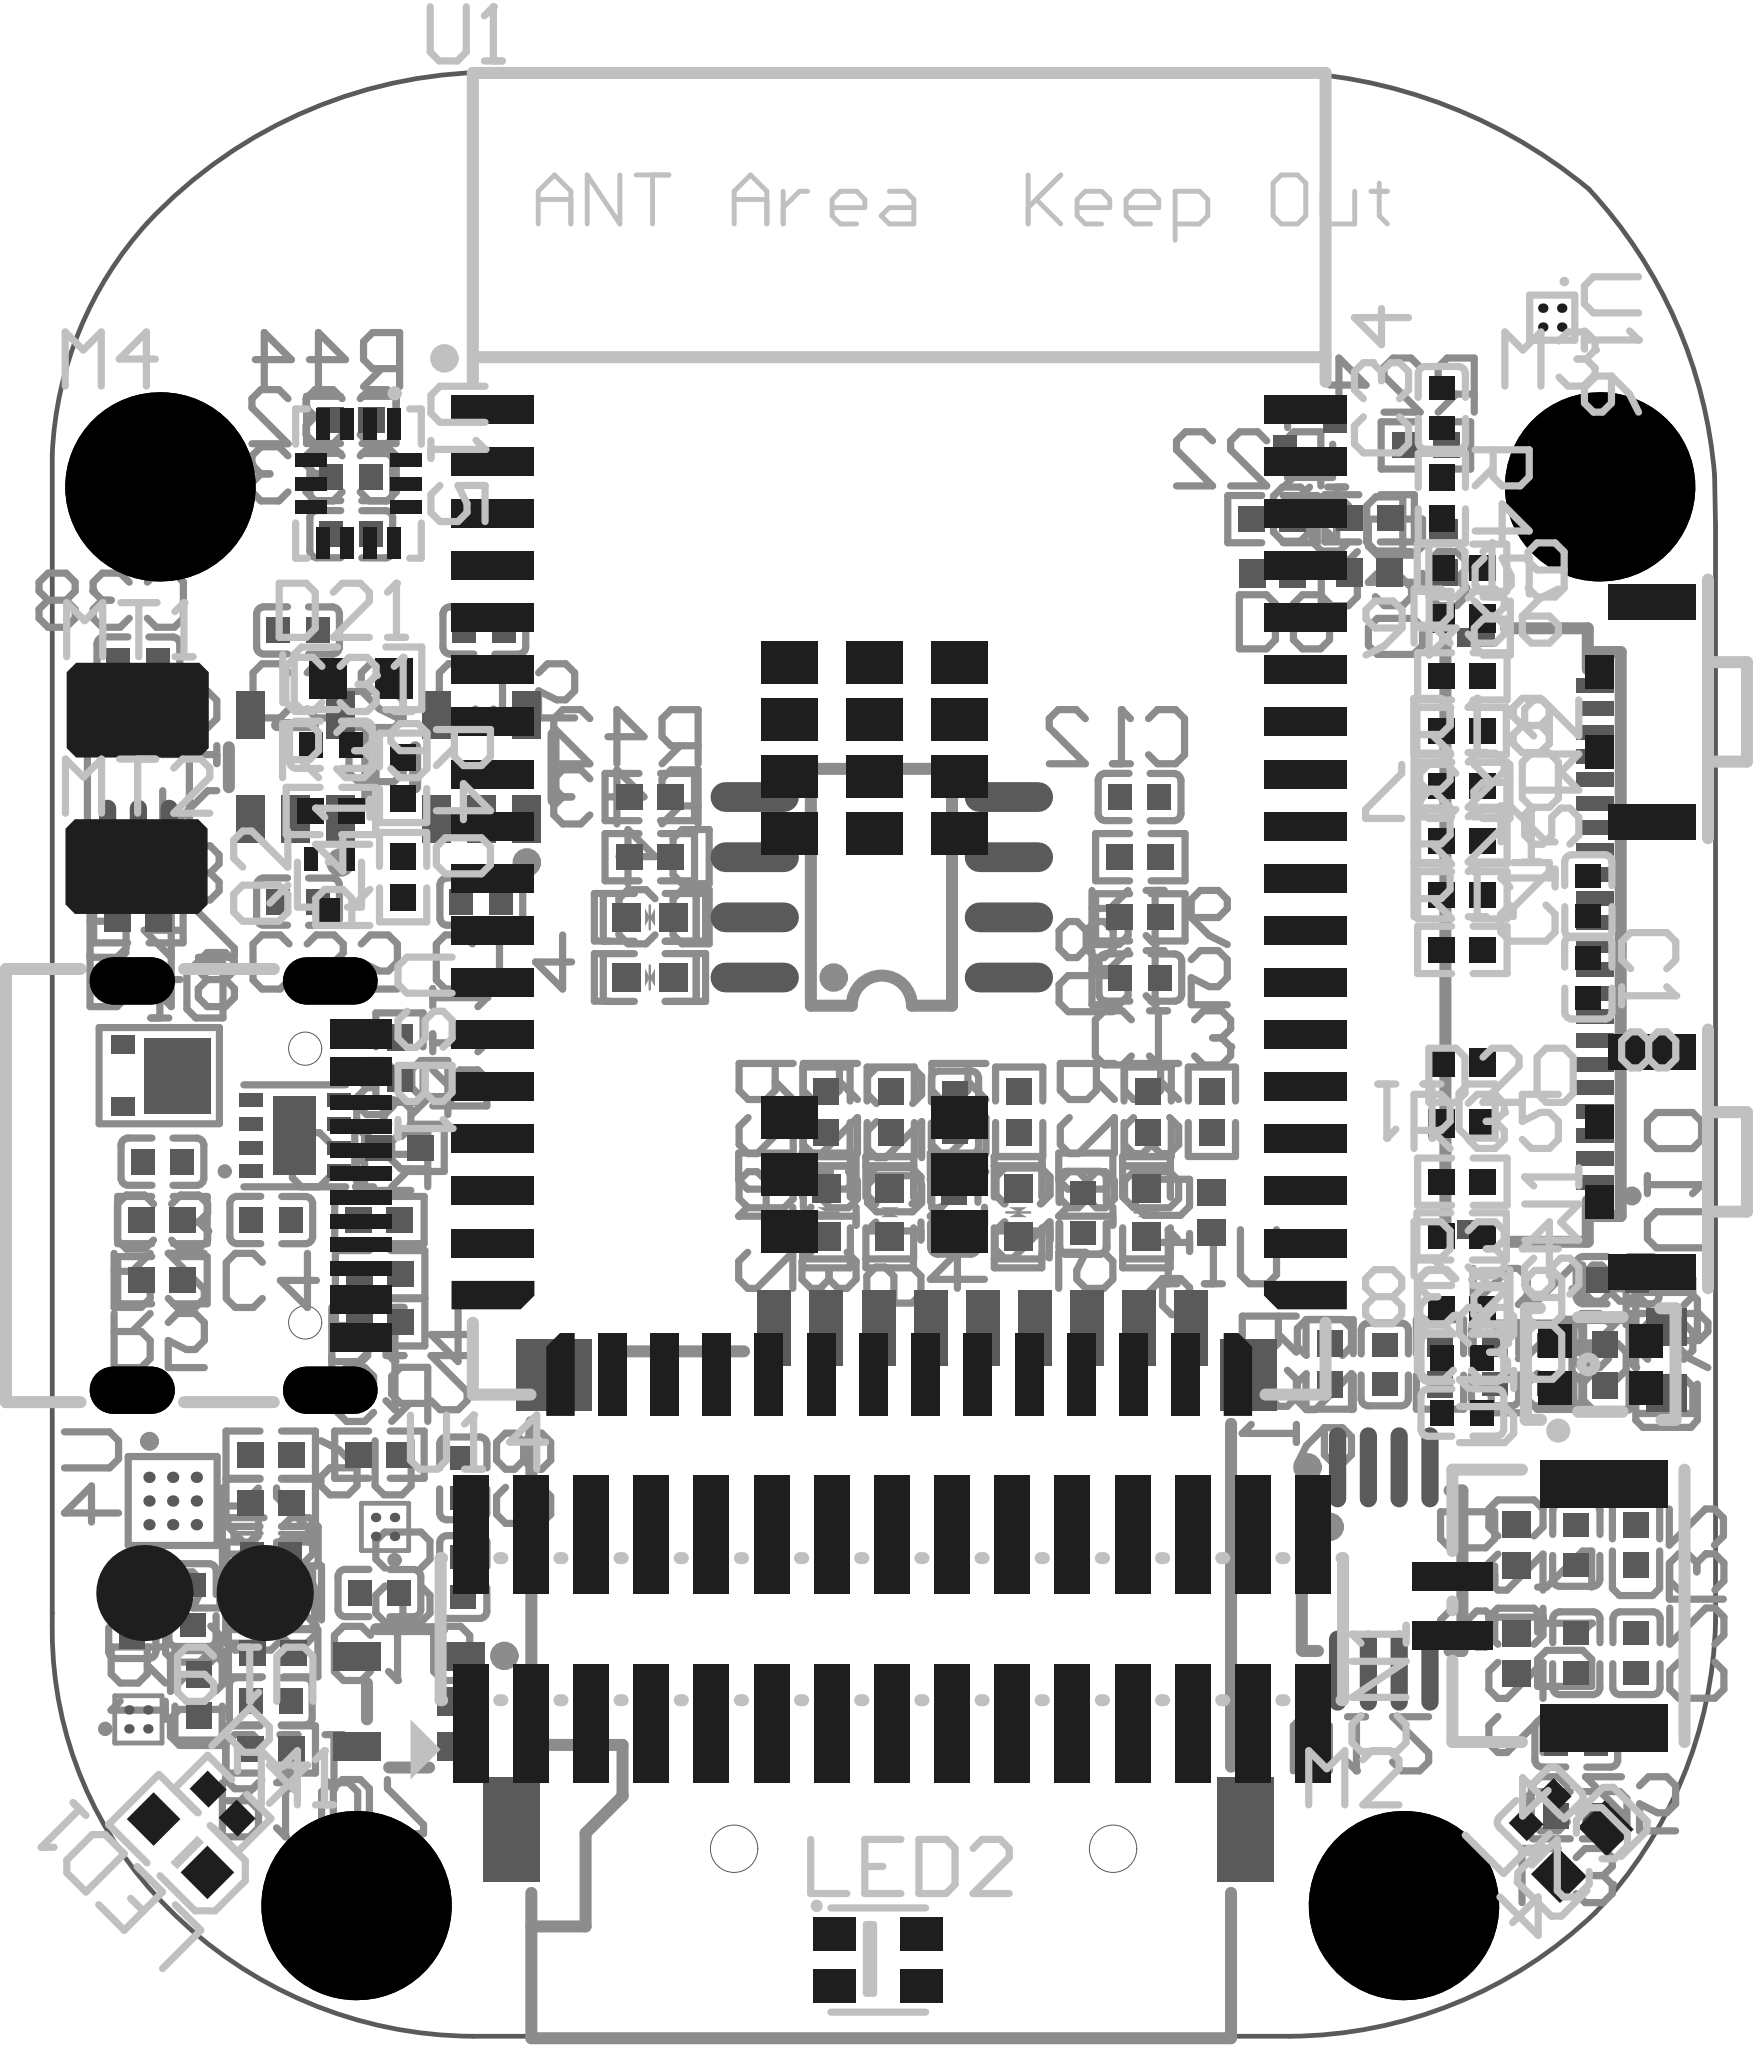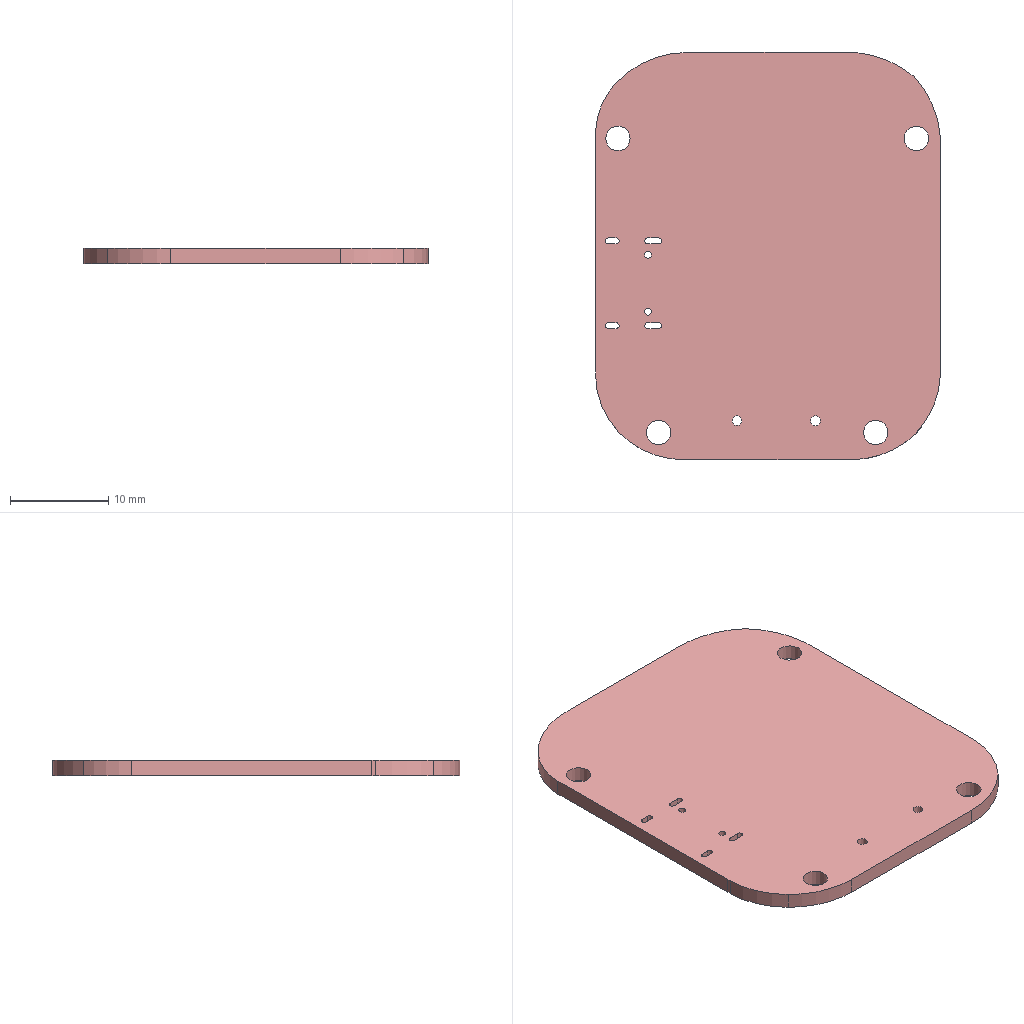Circuit board layout | Altium Designer | box 35.1 x 41.5 x 1.6 mm
Layer stack:
# Altium Designer layer stack of  (unit mm; dielectric type: 0 none, 1 core, 2 prepreg, 3 surface material)
index,name,kind,layer,copper_thickness_mm,dielectric_type,dielectric_thickness_mm,dielectric_material,dielectric_constant
0,Top Paste Mask Layer,other,,,,,,
1,Top Silkscreen Layer,other,,,,,,
2,Top Solder Mask Layer,dielectric,,,3,0.01,,3.3
3,Top Layer,copper,Top Layer,0.035,,,,
4,Dielectric1,dielectric,,,3,1.51,FR4,4.5
5,Bottom Layer,copper,Bottom Layer,0.035,,,,
6,Bottom Solder Mask Layer,dielectric,,,3,0.01,,3.3
7,Bottom Silkscreen Layer,other,,,,,,
8,Bottom Paste Mask Layer,other,,,,,,
# drill layer pairs: low layer,high layer
drill_pair,Top Layer,Bottom Layer
Part placement:
Designator,Comment,Layer,Footprint,Center-X(mm),Center-Y(mm),Rotation
C1,1uF,BottomLayer,C0402,98.943,93.625,270
C2,4.7uF,BottomLayer,C0402,98.926,93.625,270
C3,1uF,BottomLayer,C0402,79.502,94.704,0
C4,4.7uF,BottomLayer,C0402,81.799,93.472,0
C5,10uF,BottomLayer,C0402,78.867,85.09,90
C6,4.7uF,BottomLayer,C0402,80.137,85.344,90
C7,1uF,BottomLayer,C0402,81.839,85.344,180
C8,1uF,BottomLayer,C0402,85.852,88.019,90
C9,1uF,BottomLayer,C0402,85.852,85.936,270
C10,1uF,BottomLayer,C0402,84.082,85.598,0
C11,1uF,BottomLayer,C0402,81.788,83.312,0
C12,1uF,BottomLayer,C0402,100.128,102.402,180
C13,100nF,BottomLayer,C0402,100.144,98.592,0
C14,1uF,BottomLayer,C0402,86.233,100.194,0
C15,1uF,BottomLayer,C0402,86.297,105.918,0
C16,1uF,BottomLayer,C0402,110.218,92.202,0
C17,100nF,TopLayer,C0402,109.601,100.31,90
C18,4.7uF,TopLayer,C0402,109.601,98.59,270
C19,1uF,BottomLayer,C0402,96.216,93.625,270
C20,100nF,BottomLayer,C0402,96.231,95.743,270
C21,330pF,BottomLayer,C0402,109.347,86.614,270
C22,330pF,BottomLayer,C0402,109.347,84.328,270
C23,330pF,BottomLayer,C0402,110.617,84.328,90
C24,100nF,TopLayer,C0402,108.585,81.026,225
C25,22uF,BottomLayer,C0402,109.347,82.423,0
C26,1uF,BottomLayer,C0402,105.304,90.424,270
C27,100nF,BottomLayer,C0402,107.633,90.424,90
C28,100nF,BottomLayer,C0402,108.798,90.424,90
C29,4.7uF,TopLayer,C0402,106.942,90.563,0
C30,10nF,TopLayer,C0402,106.942,89.408,0
C31,4.7uF,TopLayer,C0402,83.058,103.505,0
C32,100nF,BottomLayer,C0402,83.488,109.157,180
C33,100nF,BottomLayer,C0402,83.488,107.95,180
C34,100nF,TopLayer,C0402,106.509,110.617,90
CN1,A1257WR-S-2P,TopLayer,CONN-SMD_A1257WR-S-2P,108.331,85.328,90
D1,PTVSHC3N18VU,BottomLayer,DFN-3_L2.0-W2.0-P1.30-BR,79.248,96.52,180
D2,PESDHC2FD12VU,BottomLayer,DFN1006-2L-RD,81.788,86.36,0
D3,,BottomLayer,D0402-BI,89.789,98.592,180
D4,,BottomLayer,D0402-BI,89.789,99.862,180
D8,ESD5451N,BottomLayer,DFN1006-2L-BI,102.934,107.125,0
D9,ESD5451N,BottomLayer,DFN1006-2L-BI,104.984,107.143,180
D10,ESD5451N,BottomLayer,DFN1006-2L-BI,106.553,107.569,270
D11,ESD5451N,TopLayer,DFN1006-2L-BI,106.934,96.796,180
D12,,BottomLayer,D0402-BI,93.519,93.633,270
D13,,BottomLayer,D0402-BI,94.855,93.633,270
D14,,BottomLayer,D0402-BI,97.565,93.633,270
D15,,BottomLayer,D0402-BI,100.275,93.633,270
D16,ESD5451N,BottomLayer,DFN1006-2L-BI,101.636,93.633,270
D17,ESD5451N,BottomLayer,DFN1006-2L-BI,108.077,84.328,90
D18,ESD5451N,BottomLayer,DFN1006-2L-BI,108.077,86.614,270
D19,ESD5451N,TopLayer,DFN1006-2L-BI,106.934,106.172,0
D20,ESD5451N,TopLayer,DFN1006-2L-BI,106.934,95.505,0
D21,CD4148WTP,TopLayer,D0603-RD,83.693,104.902,0
L2,,BottomLayer,L0402,110.617,86.614,90
L3,,BottomLayer,L0402,109.347,80.899,0
L4,,TopLayer,L0603,109.474,80.137,45
L5,,BottomLayer,L0603,111.252,90.52,270
LED1,,TopLayer,LED0603-RD_GREEN,79.883,80.264,135
LED2,WS2812B-2020,TopLayer,LED-SMD_4P-L2.0-W2.0-TL_WS2812B-2020,94.613,77.851,0
Q1,CJ3134K KF,BottomLayer,SOT-723_L1.2-W0.8-P0.40-LS1.2-BR,103.729,109.825,0
Q2,CJ3134K KF,TopLayer,SOT-723_L1.2-W0.8-P0.40-LS1.2-BR,83.028,100.554,90
R1,100kΩ,BottomLayer,R0402,80.264,83.439,270
R2,510kΩ,BottomLayer,R0402,79.502,93.472,0
R3,20kΩ,BottomLayer,R0402,84.506,94.996,180
R4,4.7kΩ,TopLayer,R0402,80.772,81.153,315
R5,100kΩ,BottomLayer,R0402,79.502,92.202,0
R6,100kΩ,BottomLayer,R0402,81.839,84.328,180
R7,2.2kΩ,BottomLayer,R0402,81.788,88.519,0
R8,2.2kΩ,BottomLayer,R0402,81.788,87.503,0
R9,5.1MΩ,BottomLayer,R0402,84.082,88.519,180
R10,5.1MΩ,BottomLayer,R0402,81.788,82.296,0
R11,5.1kΩ,BottomLayer,R0402,84.506,96.901,90
R12,5.1kΩ,BottomLayer,R0402,84.097,91.313,0
R13,390kΩ,BottomLayer,R0402,84.082,93.472,180
R14,510kΩ,BottomLayer,R0402,84.097,92.329,0
R15,100Ω,BottomLayer,R0402,100.144,99.862,0
R16,100Ω,BottomLayer,R0402,100.144,101.132,0
R17,22Ω,TopLayer,R0402,106.942,99.174,0
R18,22Ω,TopLayer,R0402,106.942,102.639,0
R19,22Ω,TopLayer,R0402,106.942,102.639,0
R20,22Ω,TopLayer,R0402,106.942,101.484,0
R21,22Ω,TopLayer,R0402,106.942,100.329,0
R22,2.2kΩ,BottomLayer,R0402,102.934,108.268,180
R23,2.2kΩ,BottomLayer,R0402,104.984,108.286,0
R24,2.2kΩ,BottomLayer,R0402,106.172,109.825,180
R25,22Ω,BottomLayer,R0402,94.875,95.758,270
R27,22Ω,BottomLayer,R0402,97.587,95.758,270
R28,22Ω,BottomLayer,R0402,100.299,95.758,270
R29,22Ω,BottomLayer,R0402,93.519,95.758,270
R30,22Ω,BottomLayer,R0402,101.655,95.758,270
R31,5.1MΩ,BottomLayer,R0402,104.14,90.424,270
R32,43.2kΩ,BottomLayer,R0402,106.469,90.424,90
R33,43.2kΩ,BottomLayer,R0402,109.962,90.409,90
R34,1kΩ,TopLayer,R0402,106.942,91.591,0
R35,5.1kΩ,TopLayer,R0402,106.942,94.282,0
R36,5.1kΩ,TopLayer,R0402,106.942,104.949,0
R37,15kΩ,TopLayer,R0402,106.926,103.794,180
R38,15kΩ,TopLayer,R0402,106.926,93.127,180
R39,5.1Ω,TopLayer,R0402,83.058,102.108,0
R40,1.5MΩ,TopLayer,R0402,84.582,102.807,270
R41,1kΩ,TopLayer,R0402,84.582,100.711,90
R42,22Ω,BottomLayer,R0402,89.789,102.402,180
R43,22Ω,BottomLayer,R0402,89.789,101.132,180
R44,2.2kΩ,BottomLayer,R0402,83.488,110.363,180
R45,2.2kΩ,TopLayer,R0402,106.509,108.712,270
R46,2.2kΩ,TopLayer,R0402,106.934,107.243,180
SW1,,TopLayer,KEY-SMD_GT-TC191A-H026-L60,110.389,94.7,90
SW2,,TopLayer,KEY-SMD_GT-TC191A-H026-L60,110.389,104.2,90
U1,,TopLayer,COMM-SMD_L27.9-W18.0-P1.10_SF32LB52-MOD-1-N16R8,95.054,100.384,0
U2,LP5240HVF,BottomLayer,WLCSP-4_L0.8-W0.8-R2-C2-P0.40-BL,78.994,82.931,90
U3,LP5305AQVF,BottomLayer,DFN-8_L2.0-W2.0-P0.50-BL-EP,82.296,95.25,90
U4,AW32001ECSR,BottomLayer,WLCSP-9_L1.7-W1.7-R3-C3-P0.50-TL,79.718,87.541,270
U6,LP5240HVF,BottomLayer,WLCSP-4_L0.8-W0.8-R2-C2-P0.40-BL,84.201,86.994,180
U7,ETA5055V330DS2F,BottomLayer,SOT-23-5_L2.9-W1.6-P0.95-LS2.8-BR,84.709,83.312,0
U8,CH340N,BottomLayer,SOP-8_L4.9-W3.9-P1.27-LS6.0-BL,94.687,100.497,90
U9,ETA5055V330DS2F,BottomLayer,SOT-23-5_L2.9-W1.6-P0.95-LS2.8-BR,86.233,103.031,270
U10,AFH34-S22FIA-1H,BottomLayer,FPC-SMD_22P-P0.50_JS_AFH34-S22FIA-1H,108.489,99.513,90
U11,TF-115Y-ACP9,BottomLayer,SIM-SMD_TF-115Y-BCP9,94.644,85.9,180
U12,NS4150B,BottomLayer,MSOP-8_L3.0-W3.0-P0.65-LS5.0-BL,105.283,86.106,0
U13,LMA2718T421-OA5,TopLayer,MIC-SMD_4P-L2.8-W1.9-P1.01-TL,109.855,90.424,90
U14,XDZ127-2-15-S-1.0-G1,TopLayer,HDR-SMD_30P-P1.27-V-M-R2-C15-LS5.5_1,94.899,84.836,0
U15,LSM6DS3TR-C,TopLayer,LGA-14_L3.0-W2.5-P0.50-TL,83.64,109.019,270
U16,MMC5603NJ,TopLayer,FLIPCHIP-4_L0.8-W0.8-R2-C2-P0.40-TL,108.839,112.522,270
U17,ETA5055V330DS2F,BottomLayer,SOT-23-5_L2.9-W1.6-P0.95-LS2.8-BR,82.301,103.031,270
USB1,KH-TYPE-C-16P,TopLayer,USB-C-SMD_KH-TYPE-C-16P,81.28,94.2,270
C35,1uF,BottomLayer,C0402,82.364,100.194,0
C36,1uF,BottomLayer,C0402,82.364,105.918,0
C38,100nF,BottomLayer,C0402,78.994,105.283,180
R47,5.1MΩ,BottomLayer,R0402,78.994,100.863,0
R48,22Ω,BottomLayer,R0402,78.994,99.822,0
U18,LTR-303ALS-01,BottomLayer,TDFN-6_L2.0-W2.0-P0.65-BL,78.994,102.921,0
U19,,TopLayer,焊盘,80.391,85.598,180
M1,M2-TH,TopLayer,M2_TH_4_2.5MM,83.589,79,0
M2,M2-TH,TopLayer,M2_TH_4_2.5MM,105.699,79,0
M3,M2-TH,TopLayer,M2_TH_4_2.5MM,109.839,108.95,0
M4,M2-TH,TopLayer,M2_TH_4_2.5MM,79.449,108.95,0
MT1,,TopLayer,TP-3x2MM,78.98,104.236,0
MT2,,TopLayer,TP-3x2MM,78.955,100.934,0
Pad and via stacks:
# Altium Designer via and pad stacks of  (unit mm). Each distinct definition once, with the count of objects using it.
# via: kind,start_layer,end_layer,hole_mm,diameter_mm,mode(0 simple;1 top-mid-bottom;2 full stack),diameter_per_layer,count,example_net
# pad: kind,layer,hole_mm,hole_type(0 round;1 square;2 slot),plating,top_size,top_shape(1 round;2 rect;3 octagon;9 rounded rect),mid_size,bottom_size,mode,footprint,size_per_layer,count,example
pad,Bottom Layer,0,0,plated,0.5x0.54,2,0.5x0.54,0.5x0.54,0,C0402,,60,C1.2
pad,Bottom Layer,0,0,plated,1.6x1.4,2,1.6x1.4,1.6x1.4,0,DFN-3_L2.0-W2.0-P1.30-BR,,1,D1.3
pad,Bottom Layer,0,0,plated,0.4x0.5,2,0.4x0.5,0.4x0.5,0,DFN-3_L2.0-W2.0-P1.30-BR,,2,D1.2
pad,Bottom Layer,0,0,plated,0.5x0.6,2,0.5x0.6,0.5x0.6,0,DFN1006-2L-RD,,2,D2.1
pad,Bottom Layer,0,0,plated,0.6x0.6,2,0.6x0.6,0.6x0.6,0,D0402-BI,,12,D3.1
pad,Bottom Layer,0,0,plated,0.55x0.6,2,0.55x0.6,0.55x0.6,0,DFN1006-2L-BI,,12,D8.1
pad,Bottom Layer,0,0,plated,0.54x0.54,2,0.54x0.54,0.54x0.54,0,L0402,,4,L2.2
pad,Bottom Layer,0,0,plated,0.8x0.864,2,0.8x0.864,0.8x0.864,0,L0603,,2,L5.1
pad,Bottom Layer,0,0,plated,0.489x0.294,2,0.489x0.294,0.489x0.294,0,SOT-723_L1.2-W0.8-P0.40-LS1.2-BR,,2,Q1.1
pad,Bottom Layer,0,0,plated,0.489x0.434,2,0.489x0.434,0.489x0.434,0,SOT-723_L1.2-W0.8-P0.40-LS1.2-BR,,1,Q1.3
pad,Bottom Layer,0,0,plated,0.5657x0.54,2,0.5657x0.54,0.5657x0.54,0,R0402,,62,R1.2
pad,Bottom Layer,0,0,plated,0.2x0.2,1,0.2x0.2,0.2x0.2,0,WLCSP-4_L0.8-W0.8-R2-C2-P0.40-BL,,8,U2.A1
pad,Bottom Layer,0,0,plated,0.28x0.505,2,0.28x0.505,0.28x0.505,0,DFN-8_L2.0-W2.0-P0.50-BL-EP,,8,U3.1
pad,Bottom Layer,0,0,plated,1.65x0.9,2,1.65x0.9,1.65x0.9,0,DFN-8_L2.0-W2.0-P0.50-BL-EP,,1,U3.9
pad,Bottom Layer,0,0,plated,0.24x0.24,1,0.24x0.24,0.24x0.24,0,WLCSP-9_L1.7-W1.7-R3-C3-P0.50-TL,,9,U4.A1
pad,Bottom Layer,0,0,plated,0.6x1,2,0.6x1,0.6x1,0,SOT-23-5_L2.9-W1.6-P0.95-LS2.8-BR,,15,U7.2
pad,Bottom Layer,0,0,plated,0.63x1.865,1,0.63x1.865,0.63x1.865,0,SOP-8_L4.9-W3.9-P1.27-LS6.0-BL,,8,U8.1
pad,Bottom Layer,0,0,plated,0.4x0.8,2,0.4x0.8,0.4x0.8,0,FPC-SMD_22P-P0.50_JS_AFH34-S22FIA-1H,,2,U10.24
pad,Bottom Layer,0,0,plated,0.3x0.8,2,0.3x0.8,0.3x0.8,0,FPC-SMD_22P-P0.50_JS_AFH34-S22FIA-1H,,22,U10.22
pad,Bottom Layer,0,0,plated,0.7x1.6,2,0.7x1.6,0.7x1.6,0,SIM-SMD_TF-115Y-BCP9,,9,U11.1
pad,Bottom Layer,0,0,plated,1.2x1.5,2,1.2x1.5,1.2x1.5,0,SIM-SMD_TF-115Y-BCP9,,1,U11.10
pad,Bottom Layer,0,0,plated,1.6x1.5,2,1.6x1.5,1.6x1.5,0,SIM-SMD_TF-115Y-BCP9,,1,U11.11
pad,Bottom Layer,0,0,plated,1.2x2.2,2,1.2x2.2,1.2x2.2,0,SIM-SMD_TF-115Y-BCP9,,2,U11.12
pad,Bottom Layer,0,0,plated,0.364x1.692,1,0.364x1.692,0.364x1.692,0,MSOP-8_L3.0-W3.0-P0.65-LS5.0-BL,,8,U12.1
pad,Bottom Layer,0,0,plated,0.364x0.847,1,0.364x0.847,0.364x0.847,0,TDFN-6_L2.0-W2.0-P0.65-BL,,6,U18.1
pad,Top Layer,0,0,plated,0.5x0.54,2,0.5x0.54,0.5x0.54,0,C0402,,14,C17.2
pad,Top Layer,0,0,plated,0.6x1.7,2,0.6x1.7,0.6x1.7,0,CONN-SMD_A1257WR-S-2P,,2,CN1.2
pad,Top Layer,0,0,plated,1x2.7,2,1x2.7,1x2.7,0,CONN-SMD_A1257WR-S-2P,,2,CN1.3
pad,Top Layer,0,0,plated,0.55x0.6,2,0.55x0.6,0.55x0.6,0,DFN1006-2L-BI,,6,D11.1
pad,Top Layer,0,0,plated,0.8x0.864,2,0.8x0.864,0.8x0.864,0,D0603-RD,,2,D21.1
pad,Top Layer,0,0,plated,0.8x0.864,2,0.8x0.864,0.8x0.864,0,L0603,,2,L4.1
pad,Top Layer,0,0,plated,0.8x0.8,2,0.8x0.8,0.8x0.8,0,LED0603-RD_GREEN,,2,LED1.1
pad,Top Layer,0,0,plated,0.9x0.7,2,0.9x0.7,0.9x0.7,0,LED-SMD_4P-L2.0-W2.0-TL_WS2812B-2020,,4,LED2.1
pad,Top Layer,0,0,plated,0.489x0.294,2,0.489x0.294,0.489x0.294,0,SOT-723_L1.2-W0.8-P0.40-LS1.2-BR,,2,Q2.1
pad,Top Layer,0,0,plated,0.489x0.434,2,0.489x0.434,0.489x0.434,0,SOT-723_L1.2-W0.8-P0.40-LS1.2-BR,,1,Q2.3
pad,Top Layer,0,0,plated,0.5657x0.54,2,0.5657x0.54,0.5657x0.54,0,R0402,,32,R4.2
pad,Top Layer,0,0,plated,0.7x0.6,2,0.7x0.6,0.7x0.6,0,KEY-SMD_GT-TC191A-H026-L60,,4,SW1.2
pad,Top Layer,0,0,plated,0.75x1.85,2,0.75x1.85,0.75x1.85,0,KEY-SMD_GT-TC191A-H026-L60,,4,SW1.3
pad,Top Layer,0,0,plated,1.75x0.6,2,1.75x0.6,1.75x0.6,0,COMM-SMD_L27.9-W18.0-P1.10_SF32LB52-MOD-1-N16R8,,46,U1.1
pad,Top Layer,0,0,plated,1.2x0.9,2,1.2x0.9,1.2x0.9,0,COMM-SMD_L27.9-W18.0-P1.10_SF32LB52-MOD-1-N16R8,,18,U1.49
pad,Top Layer,0,0,plated,0.2915x0.2915,1,0.2915x0.2915,0.2915x0.2915,0,COMM-SMD_L27.9-W18.0-P1.10_SF32LB52-MOD-1-N16R8,,4,U1.31
pad,Top Layer,0,0,plated,0.7x0.7,2,0.7x0.7,0.7x0.7,0,MIC-SMD_4P-L2.8-W1.9-P1.01-TL,,4,U13.1
pad,Top Layer,0,0,plated,0.74x2.5,2,0.74x2.5,0.74x2.5,0,HDR-SMD_30P-P1.27-V-M-R2-C15-LS5.5_1,,30,U14.30
pad,Top Layer,0,0,plated,0.675x0.28,2,0.675x0.28,0.675x0.28,0,LGA-14_L3.0-W2.5-P0.50-TL,,8,U15.1
pad,Top Layer,0,0,plated,0.28x0.675,2,0.28x0.675,0.28x0.675,0,LGA-14_L3.0-W2.5-P0.50-TL,,6,U15.5
pad,Top Layer,0,0,plated,0.2x0.2,1,0.2x0.2,0.2x0.2,0,FLIPCHIP-4_L0.8-W0.8-R2-C2-P0.40-TL,,4,U16.A1
pad,Top Layer,0,0,plated,0.3x1.3,2,0.3x1.3,0.3x1.3,0,USB-C-SMD_KH-TYPE-C-16P,,16,USB1.A1
pad,Top Layer,0,0,plated,2.032x2.032,1,2.032x2.032,2.032x2.032,0,\u00BA\u00B8\u00C5\u00CC,,2,U19.1
pad,Top Layer,0,0,plated,1x1,1,1x1,1x1,0,TP-3x2MM,,2,MT1.1
pad,Multi-Layer,0.6,2,plated,1x1.8,1,1x1.8,1x1.8,0,USB-C-SMD_KH-TYPE-C-16P,,2,USB1.3
pad,Multi-Layer,0.6,2,plated,1x2,1,1x2,1x2,0,USB-C-SMD_KH-TYPE-C-16P,,2,USB1.2
pad,Multi-Layer,2.5,0,plated,4x4,1,4x4,4x4,0,M2_TH_4_2.5MM,,4,M1.1